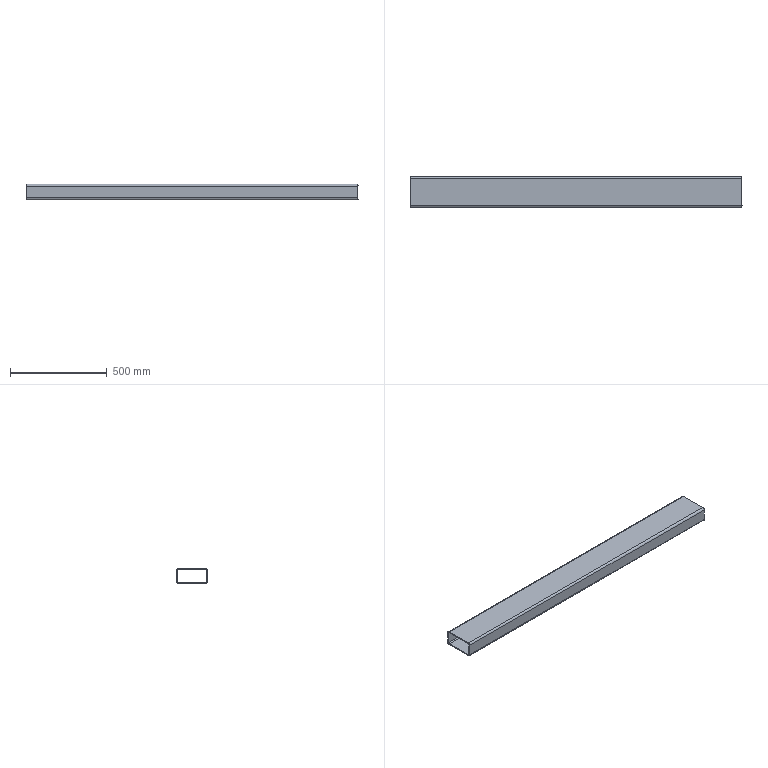Part | SolidWorks | features BaseBody 1 | 1 solid | 18 faces | box 1720 x 160 x 80 mm | volume 3845265 mm3 | plane 10 | cylinder 8 | commonest cylinder face diameters 10 x4 20 x4
STEP:
#1=CARTESIAN_POINT('',(-860.,70.,-40.));
#2=VERTEX_POINT('',#1);
#3=CARTESIAN_POINT('',(-860.,80.,-30.));
#4=VERTEX_POINT('',#3);
#5=CARTESIAN_POINT('',(-860.,70.,-30.));
#6=DIRECTION('',(1.,0.,0.));
#7=DIRECTION('',(0.,0.,-1.));
#8=AXIS2_PLACEMENT_3D('',#5,#6,#7);
#9=CIRCLE('',#8,10.);
#10=EDGE_CURVE('',#2,#4,#9,.T.);
#11=ORIENTED_EDGE('',*,*,#10,.T.);
#12=CARTESIAN_POINT('',(860.,80.,-30.));
#13=VERTEX_POINT('',#12);
#14=CARTESIAN_POINT('',(860.,80.,-30.));
#15=DIRECTION('',(-1.,0.,0.));
#16=VECTOR('',#15,1000.);
#17=LINE('',#14,#16);
#18=EDGE_CURVE('',#13,#4,#17,.T.);
#19=ORIENTED_EDGE('',*,*,#18,.F.);
#20=CARTESIAN_POINT('',(860.,70.,-40.));
#21=VERTEX_POINT('',#20);
#22=CARTESIAN_POINT('',(860.,70.,-30.));
#23=DIRECTION('',(1.,0.,0.));
#24=DIRECTION('',(0.,0.,-1.));
#25=AXIS2_PLACEMENT_3D('',#22,#23,#24);
#26=CIRCLE('',#25,10.);
#27=EDGE_CURVE('',#21,#13,#26,.T.);
#28=ORIENTED_EDGE('',*,*,#27,.F.);
#29=CARTESIAN_POINT('',(860.,70.,-40.));
#30=DIRECTION('',(-1.,0.,0.));
#31=VECTOR('',#30,1000.);
#32=LINE('',#29,#31);
#33=EDGE_CURVE('',#21,#2,#32,.T.);
#34=ORIENTED_EDGE('',*,*,#33,.T.);
#35=EDGE_LOOP('',(#11,#19,#28,#34));
#36=FACE_OUTER_BOUND('',#35,.T.);
#37=CARTESIAN_POINT('',(860.,70.,-30.));
#38=DIRECTION('',(-1.,0.,0.));
#39=DIRECTION('',(0.,0.,1.));
#40=AXIS2_PLACEMENT_3D('',#37,#38,#39);
#41=CYLINDRICAL_SURFACE('',#40,10.);
#42=ADVANCED_FACE('',(#36),#41,.T.);
#43=CARTESIAN_POINT('',(-860.,80.,30.));
#44=VERTEX_POINT('',#43);
#45=CARTESIAN_POINT('',(-860.,80.,-30.));
#46=DIRECTION('',(0.,0.,1.));
#47=VECTOR('',#46,1000.);
#48=LINE('',#45,#47);
#49=EDGE_CURVE('',#4,#44,#48,.T.);
#50=ORIENTED_EDGE('',*,*,#49,.T.);
#51=CARTESIAN_POINT('',(860.,80.,30.));
#52=VERTEX_POINT('',#51);
#53=CARTESIAN_POINT('',(860.,80.,30.));
#54=DIRECTION('',(-1.,0.,0.));
#55=VECTOR('',#54,1000.);
#56=LINE('',#53,#55);
#57=EDGE_CURVE('',#52,#44,#56,.T.);
#58=ORIENTED_EDGE('',*,*,#57,.F.);
#59=CARTESIAN_POINT('',(860.,80.,-30.));
#60=DIRECTION('',(0.,0.,1.));
#61=VECTOR('',#60,1000.);
#62=LINE('',#59,#61);
#63=EDGE_CURVE('',#13,#52,#62,.T.);
#64=ORIENTED_EDGE('',*,*,#63,.F.);
#65=ORIENTED_EDGE('',*,*,#18,.T.);
#66=EDGE_LOOP('',(#50,#58,#64,#65));
#67=FACE_OUTER_BOUND('',#66,.T.);
#68=CARTESIAN_POINT('',(860.,80.,-30.));
#69=DIRECTION('',(0.,-1.,0.));
#70=DIRECTION('',(0.,0.,-1.));
#71=AXIS2_PLACEMENT_3D('',#68,#69,#70);
#72=PLANE('',#71);
#73=ADVANCED_FACE('',(#67),#72,.F.);
#74=CARTESIAN_POINT('',(-860.,70.,40.));
#75=VERTEX_POINT('',#74);
#76=CARTESIAN_POINT('',(-860.,70.,30.));
#77=DIRECTION('',(1.,0.,0.));
#78=DIRECTION('',(0.,0.,-1.));
#79=AXIS2_PLACEMENT_3D('',#76,#77,#78);
#80=CIRCLE('',#79,10.);
#81=EDGE_CURVE('',#44,#75,#80,.T.);
#82=ORIENTED_EDGE('',*,*,#81,.T.);
#83=CARTESIAN_POINT('',(860.,70.,40.));
#84=VERTEX_POINT('',#83);
#85=CARTESIAN_POINT('',(860.,70.,40.));
#86=DIRECTION('',(-1.,0.,0.));
#87=VECTOR('',#86,1000.);
#88=LINE('',#85,#87);
#89=EDGE_CURVE('',#84,#75,#88,.T.);
#90=ORIENTED_EDGE('',*,*,#89,.F.);
#91=CARTESIAN_POINT('',(860.,70.,30.));
#92=DIRECTION('',(1.,0.,0.));
#93=DIRECTION('',(0.,0.,-1.));
#94=AXIS2_PLACEMENT_3D('',#91,#92,#93);
#95=CIRCLE('',#94,10.);
#96=EDGE_CURVE('',#52,#84,#95,.T.);
#97=ORIENTED_EDGE('',*,*,#96,.F.);
#98=ORIENTED_EDGE('',*,*,#57,.T.);
#99=EDGE_LOOP('',(#82,#90,#97,#98));
#100=FACE_OUTER_BOUND('',#99,.T.);
#101=CARTESIAN_POINT('',(860.,70.,30.));
#102=DIRECTION('',(-1.,0.,0.));
#103=DIRECTION('',(0.,0.,1.));
#104=AXIS2_PLACEMENT_3D('',#101,#102,#103);
#105=CYLINDRICAL_SURFACE('',#104,10.);
#106=ADVANCED_FACE('',(#100),#105,.T.);
#107=CARTESIAN_POINT('',(-860.,-70.,40.));
#108=VERTEX_POINT('',#107);
#109=CARTESIAN_POINT('',(-860.,-70.,40.));
#110=DIRECTION('',(0.,-1.,0.));
#111=VECTOR('',#110,1000.);
#112=LINE('',#109,#111);
#113=EDGE_CURVE('',#75,#108,#112,.T.);
#114=ORIENTED_EDGE('',*,*,#113,.T.);
#115=CARTESIAN_POINT('',(860.,-70.,40.));
#116=VERTEX_POINT('',#115);
#117=CARTESIAN_POINT('',(860.,-70.,40.));
#118=DIRECTION('',(-1.,0.,0.));
#119=VECTOR('',#118,1000.);
#120=LINE('',#117,#119);
#121=EDGE_CURVE('',#116,#108,#120,.T.);
#122=ORIENTED_EDGE('',*,*,#121,.F.);
#123=CARTESIAN_POINT('',(860.,-70.,40.));
#124=DIRECTION('',(0.,-1.,0.));
#125=VECTOR('',#124,1000.);
#126=LINE('',#123,#125);
#127=EDGE_CURVE('',#84,#116,#126,.T.);
#128=ORIENTED_EDGE('',*,*,#127,.F.);
#129=ORIENTED_EDGE('',*,*,#89,.T.);
#130=EDGE_LOOP('',(#114,#122,#128,#129));
#131=FACE_OUTER_BOUND('',#130,.T.);
#132=CARTESIAN_POINT('',(860.,-70.,40.));
#133=DIRECTION('',(0.,0.,-1.));
#134=DIRECTION('',(0.,1.,0.));
#135=AXIS2_PLACEMENT_3D('',#132,#133,#134);
#136=PLANE('',#135);
#137=ADVANCED_FACE('',(#131),#136,.F.);
#138=CARTESIAN_POINT('',(-860.,-80.,30.));
#139=VERTEX_POINT('',#138);
#140=CARTESIAN_POINT('',(-860.,-70.,30.));
#141=DIRECTION('',(1.,0.,0.));
#142=DIRECTION('',(0.,0.,-1.));
#143=AXIS2_PLACEMENT_3D('',#140,#141,#142);
#144=CIRCLE('',#143,10.);
#145=EDGE_CURVE('',#108,#139,#144,.T.);
#146=ORIENTED_EDGE('',*,*,#145,.T.);
#147=CARTESIAN_POINT('',(860.,-80.,30.));
#148=VERTEX_POINT('',#147);
#149=CARTESIAN_POINT('',(860.,-80.,30.));
#150=DIRECTION('',(-1.,0.,0.));
#151=VECTOR('',#150,1000.);
#152=LINE('',#149,#151);
#153=EDGE_CURVE('',#148,#139,#152,.T.);
#154=ORIENTED_EDGE('',*,*,#153,.F.);
#155=CARTESIAN_POINT('',(860.,-70.,30.));
#156=DIRECTION('',(1.,0.,0.));
#157=DIRECTION('',(0.,0.,-1.));
#158=AXIS2_PLACEMENT_3D('',#155,#156,#157);
#159=CIRCLE('',#158,10.);
#160=EDGE_CURVE('',#116,#148,#159,.T.);
#161=ORIENTED_EDGE('',*,*,#160,.F.);
#162=ORIENTED_EDGE('',*,*,#121,.T.);
#163=EDGE_LOOP('',(#146,#154,#161,#162));
#164=FACE_OUTER_BOUND('',#163,.T.);
#165=CARTESIAN_POINT('',(860.,-70.,30.));
#166=DIRECTION('',(-1.,0.,0.));
#167=DIRECTION('',(0.,0.,1.));
#168=AXIS2_PLACEMENT_3D('',#165,#166,#167);
#169=CYLINDRICAL_SURFACE('',#168,10.);
#170=ADVANCED_FACE('',(#164),#169,.T.);
#171=CARTESIAN_POINT('',(-860.,-80.,-30.));
#172=VERTEX_POINT('',#171);
#173=CARTESIAN_POINT('',(-860.,-80.,30.));
#174=DIRECTION('',(0.,0.,-1.));
#175=VECTOR('',#174,1000.);
#176=LINE('',#173,#175);
#177=EDGE_CURVE('',#139,#172,#176,.T.);
#178=ORIENTED_EDGE('',*,*,#177,.T.);
#179=CARTESIAN_POINT('',(860.,-80.,-30.));
#180=VERTEX_POINT('',#179);
#181=CARTESIAN_POINT('',(860.,-80.,-30.));
#182=DIRECTION('',(-1.,0.,0.));
#183=VECTOR('',#182,1000.);
#184=LINE('',#181,#183);
#185=EDGE_CURVE('',#180,#172,#184,.T.);
#186=ORIENTED_EDGE('',*,*,#185,.F.);
#187=CARTESIAN_POINT('',(860.,-80.,30.));
#188=DIRECTION('',(0.,0.,-1.));
#189=VECTOR('',#188,1000.);
#190=LINE('',#187,#189);
#191=EDGE_CURVE('',#148,#180,#190,.T.);
#192=ORIENTED_EDGE('',*,*,#191,.F.);
#193=ORIENTED_EDGE('',*,*,#153,.T.);
#194=EDGE_LOOP('',(#178,#186,#192,#193));
#195=FACE_OUTER_BOUND('',#194,.T.);
#196=CARTESIAN_POINT('',(860.,-80.,30.));
#197=DIRECTION('',(0.,1.,0.));
#198=DIRECTION('',(0.,0.,1.));
#199=AXIS2_PLACEMENT_3D('',#196,#197,#198);
#200=PLANE('',#199);
#201=ADVANCED_FACE('',(#195),#200,.F.);
#202=CARTESIAN_POINT('',(-860.,-70.,-40.));
#203=VERTEX_POINT('',#202);
#204=CARTESIAN_POINT('',(-860.,-70.,-30.));
#205=DIRECTION('',(1.,0.,0.));
#206=DIRECTION('',(0.,0.,-1.));
#207=AXIS2_PLACEMENT_3D('',#204,#205,#206);
#208=CIRCLE('',#207,10.);
#209=EDGE_CURVE('',#172,#203,#208,.T.);
#210=ORIENTED_EDGE('',*,*,#209,.T.);
#211=CARTESIAN_POINT('',(860.,-70.,-40.));
#212=VERTEX_POINT('',#211);
#213=CARTESIAN_POINT('',(860.,-70.,-40.));
#214=DIRECTION('',(-1.,0.,0.));
#215=VECTOR('',#214,1000.);
#216=LINE('',#213,#215);
#217=EDGE_CURVE('',#212,#203,#216,.T.);
#218=ORIENTED_EDGE('',*,*,#217,.F.);
#219=CARTESIAN_POINT('',(860.,-70.,-30.));
#220=DIRECTION('',(1.,0.,0.));
#221=DIRECTION('',(0.,0.,-1.));
#222=AXIS2_PLACEMENT_3D('',#219,#220,#221);
#223=CIRCLE('',#222,10.);
#224=EDGE_CURVE('',#180,#212,#223,.T.);
#225=ORIENTED_EDGE('',*,*,#224,.F.);
#226=ORIENTED_EDGE('',*,*,#185,.T.);
#227=EDGE_LOOP('',(#210,#218,#225,#226));
#228=FACE_OUTER_BOUND('',#227,.T.);
#229=CARTESIAN_POINT('',(860.,-70.,-30.));
#230=DIRECTION('',(-1.,0.,0.));
#231=DIRECTION('',(0.,0.,1.));
#232=AXIS2_PLACEMENT_3D('',#229,#230,#231);
#233=CYLINDRICAL_SURFACE('',#232,10.);
#234=ADVANCED_FACE('',(#228),#233,.T.);
#235=CARTESIAN_POINT('',(-860.,75.,30.));
#236=VERTEX_POINT('',#235);
#237=CARTESIAN_POINT('',(-860.,70.,35.));
#238=VERTEX_POINT('',#237);
#239=CARTESIAN_POINT('',(-860.,70.,30.));
#240=DIRECTION('',(1.,0.,0.));
#241=DIRECTION('',(0.,0.,-1.));
#242=AXIS2_PLACEMENT_3D('',#239,#240,#241);
#243=CIRCLE('',#242,5.);
#244=EDGE_CURVE('',#236,#238,#243,.T.);
#245=ORIENTED_EDGE('',*,*,#244,.F.);
#246=CARTESIAN_POINT('',(860.,75.,30.));
#247=VERTEX_POINT('',#246);
#248=CARTESIAN_POINT('',(860.,75.,30.));
#249=DIRECTION('',(-1.,0.,0.));
#250=VECTOR('',#249,1000.);
#251=LINE('',#248,#250);
#252=EDGE_CURVE('',#247,#236,#251,.T.);
#253=ORIENTED_EDGE('',*,*,#252,.F.);
#254=CARTESIAN_POINT('',(860.,70.,35.));
#255=VERTEX_POINT('',#254);
#256=CARTESIAN_POINT('',(860.,70.,30.));
#257=DIRECTION('',(1.,0.,0.));
#258=DIRECTION('',(0.,0.,-1.));
#259=AXIS2_PLACEMENT_3D('',#256,#257,#258);
#260=CIRCLE('',#259,5.);
#261=EDGE_CURVE('',#247,#255,#260,.T.);
#262=ORIENTED_EDGE('',*,*,#261,.T.);
#263=CARTESIAN_POINT('',(860.,70.,35.));
#264=DIRECTION('',(-1.,0.,0.));
#265=VECTOR('',#264,1000.);
#266=LINE('',#263,#265);
#267=EDGE_CURVE('',#255,#238,#266,.T.);
#268=ORIENTED_EDGE('',*,*,#267,.T.);
#269=EDGE_LOOP('',(#245,#253,#262,#268));
#270=FACE_OUTER_BOUND('',#269,.T.);
#271=CARTESIAN_POINT('',(860.,70.,30.));
#272=DIRECTION('',(-1.,0.,0.));
#273=DIRECTION('',(0.,0.,1.));
#274=AXIS2_PLACEMENT_3D('',#271,#272,#273);
#275=CYLINDRICAL_SURFACE('',#274,5.);
#276=ADVANCED_FACE('',(#270),#275,.F.);
#277=CARTESIAN_POINT('',(-860.,75.,-30.));
#278=VERTEX_POINT('',#277);
#279=CARTESIAN_POINT('',(-860.,75.,-30.));
#280=DIRECTION('',(0.,0.,1.));
#281=VECTOR('',#280,1000.);
#282=LINE('',#279,#281);
#283=EDGE_CURVE('',#278,#236,#282,.T.);
#284=ORIENTED_EDGE('',*,*,#283,.F.);
#285=CARTESIAN_POINT('',(860.,75.,-30.));
#286=VERTEX_POINT('',#285);
#287=CARTESIAN_POINT('',(860.,75.,-30.));
#288=DIRECTION('',(-1.,0.,0.));
#289=VECTOR('',#288,1000.);
#290=LINE('',#287,#289);
#291=EDGE_CURVE('',#286,#278,#290,.T.);
#292=ORIENTED_EDGE('',*,*,#291,.F.);
#293=CARTESIAN_POINT('',(860.,75.,-30.));
#294=DIRECTION('',(0.,0.,1.));
#295=VECTOR('',#294,1000.);
#296=LINE('',#293,#295);
#297=EDGE_CURVE('',#286,#247,#296,.T.);
#298=ORIENTED_EDGE('',*,*,#297,.T.);
#299=ORIENTED_EDGE('',*,*,#252,.T.);
#300=EDGE_LOOP('',(#284,#292,#298,#299));
#301=FACE_OUTER_BOUND('',#300,.T.);
#302=CARTESIAN_POINT('',(860.,75.,-30.));
#303=DIRECTION('',(0.,-1.,0.));
#304=DIRECTION('',(0.,0.,-1.));
#305=AXIS2_PLACEMENT_3D('',#302,#303,#304);
#306=PLANE('',#305);
#307=ADVANCED_FACE('',(#301),#306,.T.);
#308=CARTESIAN_POINT('',(-860.,70.,-35.));
#309=VERTEX_POINT('',#308);
#310=CARTESIAN_POINT('',(-860.,70.,-30.));
#311=DIRECTION('',(1.,0.,0.));
#312=DIRECTION('',(0.,0.,-1.));
#313=AXIS2_PLACEMENT_3D('',#310,#311,#312);
#314=CIRCLE('',#313,5.);
#315=EDGE_CURVE('',#309,#278,#314,.T.);
#316=ORIENTED_EDGE('',*,*,#315,.F.);
#317=CARTESIAN_POINT('',(860.,70.,-35.));
#318=VERTEX_POINT('',#317);
#319=CARTESIAN_POINT('',(860.,70.,-35.));
#320=DIRECTION('',(-1.,0.,0.));
#321=VECTOR('',#320,1000.);
#322=LINE('',#319,#321);
#323=EDGE_CURVE('',#318,#309,#322,.T.);
#324=ORIENTED_EDGE('',*,*,#323,.F.);
#325=CARTESIAN_POINT('',(860.,70.,-30.));
#326=DIRECTION('',(1.,0.,0.));
#327=DIRECTION('',(0.,0.,-1.));
#328=AXIS2_PLACEMENT_3D('',#325,#326,#327);
#329=CIRCLE('',#328,5.);
#330=EDGE_CURVE('',#318,#286,#329,.T.);
#331=ORIENTED_EDGE('',*,*,#330,.T.);
#332=ORIENTED_EDGE('',*,*,#291,.T.);
#333=EDGE_LOOP('',(#316,#324,#331,#332));
#334=FACE_OUTER_BOUND('',#333,.T.);
#335=CARTESIAN_POINT('',(860.,70.,-30.));
#336=DIRECTION('',(-1.,0.,0.));
#337=DIRECTION('',(0.,0.,1.));
#338=AXIS2_PLACEMENT_3D('',#335,#336,#337);
#339=CYLINDRICAL_SURFACE('',#338,5.);
#340=ADVANCED_FACE('',(#334),#339,.F.);
#341=CARTESIAN_POINT('',(-860.,-70.,-35.));
#342=VERTEX_POINT('',#341);
#343=CARTESIAN_POINT('',(-860.,70.,-35.));
#344=DIRECTION('',(0.,1.,0.));
#345=VECTOR('',#344,1000.);
#346=LINE('',#343,#345);
#347=EDGE_CURVE('',#342,#309,#346,.T.);
#348=ORIENTED_EDGE('',*,*,#347,.F.);
#349=CARTESIAN_POINT('',(860.,-70.,-35.));
#350=VERTEX_POINT('',#349);
#351=CARTESIAN_POINT('',(860.,-70.,-35.));
#352=DIRECTION('',(-1.,0.,0.));
#353=VECTOR('',#352,1000.);
#354=LINE('',#351,#353);
#355=EDGE_CURVE('',#350,#342,#354,.T.);
#356=ORIENTED_EDGE('',*,*,#355,.F.);
#357=CARTESIAN_POINT('',(860.,70.,-35.));
#358=DIRECTION('',(0.,1.,0.));
#359=VECTOR('',#358,1000.);
#360=LINE('',#357,#359);
#361=EDGE_CURVE('',#350,#318,#360,.T.);
#362=ORIENTED_EDGE('',*,*,#361,.T.);
#363=ORIENTED_EDGE('',*,*,#323,.T.);
#364=EDGE_LOOP('',(#348,#356,#362,#363));
#365=FACE_OUTER_BOUND('',#364,.T.);
#366=CARTESIAN_POINT('',(860.,70.,-35.));
#367=DIRECTION('',(0.,0.,1.));
#368=DIRECTION('',(1.,0.,0.));
#369=AXIS2_PLACEMENT_3D('',#366,#367,#368);
#370=PLANE('',#369);
#371=ADVANCED_FACE('',(#365),#370,.T.);
#372=CARTESIAN_POINT('',(-860.,-75.,-30.));
#373=VERTEX_POINT('',#372);
#374=CARTESIAN_POINT('',(-860.,-70.,-30.));
#375=DIRECTION('',(1.,0.,0.));
#376=DIRECTION('',(0.,0.,-1.));
#377=AXIS2_PLACEMENT_3D('',#374,#375,#376);
#378=CIRCLE('',#377,5.);
#379=EDGE_CURVE('',#373,#342,#378,.T.);
#380=ORIENTED_EDGE('',*,*,#379,.F.);
#381=CARTESIAN_POINT('',(860.,-75.,-30.));
#382=VERTEX_POINT('',#381);
#383=CARTESIAN_POINT('',(860.,-75.,-30.));
#384=DIRECTION('',(-1.,0.,0.));
#385=VECTOR('',#384,1000.);
#386=LINE('',#383,#385);
#387=EDGE_CURVE('',#382,#373,#386,.T.);
#388=ORIENTED_EDGE('',*,*,#387,.F.);
#389=CARTESIAN_POINT('',(860.,-70.,-30.));
#390=DIRECTION('',(1.,0.,0.));
#391=DIRECTION('',(0.,0.,-1.));
#392=AXIS2_PLACEMENT_3D('',#389,#390,#391);
#393=CIRCLE('',#392,5.);
#394=EDGE_CURVE('',#382,#350,#393,.T.);
#395=ORIENTED_EDGE('',*,*,#394,.T.);
#396=ORIENTED_EDGE('',*,*,#355,.T.);
#397=EDGE_LOOP('',(#380,#388,#395,#396));
#398=FACE_OUTER_BOUND('',#397,.T.);
#399=CARTESIAN_POINT('',(860.,-70.,-30.));
#400=DIRECTION('',(-1.,0.,0.));
#401=DIRECTION('',(0.,0.,1.));
#402=AXIS2_PLACEMENT_3D('',#399,#400,#401);
#403=CYLINDRICAL_SURFACE('',#402,5.);
#404=ADVANCED_FACE('',(#398),#403,.F.);
#405=CARTESIAN_POINT('',(-860.,-75.,30.));
#406=VERTEX_POINT('',#405);
#407=CARTESIAN_POINT('',(-860.,-75.,30.));
#408=DIRECTION('',(0.,0.,-1.));
#409=VECTOR('',#408,1000.);
#410=LINE('',#407,#409);
#411=EDGE_CURVE('',#406,#373,#410,.T.);
#412=ORIENTED_EDGE('',*,*,#411,.F.);
#413=CARTESIAN_POINT('',(860.,-75.,30.));
#414=VERTEX_POINT('',#413);
#415=CARTESIAN_POINT('',(860.,-75.,30.));
#416=DIRECTION('',(-1.,0.,0.));
#417=VECTOR('',#416,1000.);
#418=LINE('',#415,#417);
#419=EDGE_CURVE('',#414,#406,#418,.T.);
#420=ORIENTED_EDGE('',*,*,#419,.F.);
#421=CARTESIAN_POINT('',(860.,-75.,30.));
#422=DIRECTION('',(0.,0.,-1.));
#423=VECTOR('',#422,1000.);
#424=LINE('',#421,#423);
#425=EDGE_CURVE('',#414,#382,#424,.T.);
#426=ORIENTED_EDGE('',*,*,#425,.T.);
#427=ORIENTED_EDGE('',*,*,#387,.T.);
#428=EDGE_LOOP('',(#412,#420,#426,#427));
#429=FACE_OUTER_BOUND('',#428,.T.);
#430=CARTESIAN_POINT('',(860.,-75.,30.));
#431=DIRECTION('',(0.,1.,0.));
#432=DIRECTION('',(0.,0.,1.));
#433=AXIS2_PLACEMENT_3D('',#430,#431,#432);
#434=PLANE('',#433);
#435=ADVANCED_FACE('',(#429),#434,.T.);
#436=CARTESIAN_POINT('',(-860.,-70.,35.));
#437=VERTEX_POINT('',#436);
#438=CARTESIAN_POINT('',(-860.,-70.,30.));
#439=DIRECTION('',(1.,0.,0.));
#440=DIRECTION('',(0.,0.,-1.));
#441=AXIS2_PLACEMENT_3D('',#438,#439,#440);
#442=CIRCLE('',#441,5.);
#443=EDGE_CURVE('',#437,#406,#442,.T.);
#444=ORIENTED_EDGE('',*,*,#443,.F.);
#445=CARTESIAN_POINT('',(860.,-70.,35.));
#446=VERTEX_POINT('',#445);
#447=CARTESIAN_POINT('',(860.,-70.,35.));
#448=DIRECTION('',(-1.,0.,0.));
#449=VECTOR('',#448,1000.);
#450=LINE('',#447,#449);
#451=EDGE_CURVE('',#446,#437,#450,.T.);
#452=ORIENTED_EDGE('',*,*,#451,.F.);
#453=CARTESIAN_POINT('',(860.,-70.,30.));
#454=DIRECTION('',(1.,0.,0.));
#455=DIRECTION('',(0.,0.,-1.));
#456=AXIS2_PLACEMENT_3D('',#453,#454,#455);
#457=CIRCLE('',#456,5.);
#458=EDGE_CURVE('',#446,#414,#457,.T.);
#459=ORIENTED_EDGE('',*,*,#458,.T.);
#460=ORIENTED_EDGE('',*,*,#419,.T.);
#461=EDGE_LOOP('',(#444,#452,#459,#460));
#462=FACE_OUTER_BOUND('',#461,.T.);
#463=CARTESIAN_POINT('',(860.,-70.,30.));
#464=DIRECTION('',(-1.,0.,0.));
#465=DIRECTION('',(0.,0.,1.));
#466=AXIS2_PLACEMENT_3D('',#463,#464,#465);
#467=CYLINDRICAL_SURFACE('',#466,5.);
#468=ADVANCED_FACE('',(#462),#467,.F.);
#469=CARTESIAN_POINT('',(-860.,-70.,35.));
#470=DIRECTION('',(0.,-1.,0.));
#471=VECTOR('',#470,1000.);
#472=LINE('',#469,#471);
#473=EDGE_CURVE('',#238,#437,#472,.T.);
#474=ORIENTED_EDGE('',*,*,#473,.F.);
#475=ORIENTED_EDGE('',*,*,#267,.F.);
#476=CARTESIAN_POINT('',(860.,-70.,35.));
#477=DIRECTION('',(0.,-1.,0.));
#478=VECTOR('',#477,1000.);
#479=LINE('',#476,#478);
#480=EDGE_CURVE('',#255,#446,#479,.T.);
#481=ORIENTED_EDGE('',*,*,#480,.T.);
#482=ORIENTED_EDGE('',*,*,#451,.T.);
#483=EDGE_LOOP('',(#474,#475,#481,#482));
#484=FACE_OUTER_BOUND('',#483,.T.);
#485=CARTESIAN_POINT('',(860.,-70.,35.));
#486=DIRECTION('',(0.,0.,-1.));
#487=DIRECTION('',(0.,1.,0.));
#488=AXIS2_PLACEMENT_3D('',#485,#486,#487);
#489=PLANE('',#488);
#490=ADVANCED_FACE('',(#484),#489,.T.);
#491=CARTESIAN_POINT('',(-860.,70.,-40.));
#492=DIRECTION('',(0.,1.,0.));
#493=VECTOR('',#492,1000.);
#494=LINE('',#491,#493);
#495=EDGE_CURVE('',#203,#2,#494,.T.);
#496=ORIENTED_EDGE('',*,*,#495,.T.);
#497=ORIENTED_EDGE('',*,*,#33,.F.);
#498=CARTESIAN_POINT('',(860.,70.,-40.));
#499=DIRECTION('',(0.,1.,0.));
#500=VECTOR('',#499,1000.);
#501=LINE('',#498,#500);
#502=EDGE_CURVE('',#212,#21,#501,.T.);
#503=ORIENTED_EDGE('',*,*,#502,.F.);
#504=ORIENTED_EDGE('',*,*,#217,.T.);
#505=EDGE_LOOP('',(#496,#497,#503,#504));
#506=FACE_OUTER_BOUND('',#505,.T.);
#507=CARTESIAN_POINT('',(860.,70.,-40.));
#508=DIRECTION('',(0.,0.,1.));
#509=DIRECTION('',(1.,0.,0.));
#510=AXIS2_PLACEMENT_3D('',#507,#508,#509);
#511=PLANE('',#510);
#512=ADVANCED_FACE('',(#506),#511,.F.);
#513=ORIENTED_EDGE('',*,*,#261,.F.);
#514=ORIENTED_EDGE('',*,*,#297,.F.);
#515=ORIENTED_EDGE('',*,*,#330,.F.);
#516=ORIENTED_EDGE('',*,*,#361,.F.);
#517=ORIENTED_EDGE('',*,*,#394,.F.);
#518=ORIENTED_EDGE('',*,*,#425,.F.);
#519=ORIENTED_EDGE('',*,*,#458,.F.);
#520=ORIENTED_EDGE('',*,*,#480,.F.);
#521=EDGE_LOOP('',(#513,#514,#515,#516,#517,#518,#519,#520));
#522=FACE_BOUND('',#521,.T.);
#523=ORIENTED_EDGE('',*,*,#27,.T.);
#524=ORIENTED_EDGE('',*,*,#63,.T.);
#525=ORIENTED_EDGE('',*,*,#96,.T.);
#526=ORIENTED_EDGE('',*,*,#127,.T.);
#527=ORIENTED_EDGE('',*,*,#160,.T.);
#528=ORIENTED_EDGE('',*,*,#191,.T.);
#529=ORIENTED_EDGE('',*,*,#224,.T.);
#530=ORIENTED_EDGE('',*,*,#502,.T.);
#531=EDGE_LOOP('',(#523,#524,#525,#526,#527,#528,#529,#530));
#532=FACE_OUTER_BOUND('',#531,.T.);
#533=CARTESIAN_POINT('',(860.,70.,-30.));
#534=DIRECTION('',(1.,0.,0.));
#535=DIRECTION('',(0.,0.,-1.));
#536=AXIS2_PLACEMENT_3D('',#533,#534,#535);
#537=PLANE('',#536);
#538=ADVANCED_FACE('',(#522,#532),#537,.T.);
#539=ORIENTED_EDGE('',*,*,#244,.T.);
#540=ORIENTED_EDGE('',*,*,#473,.T.);
#541=ORIENTED_EDGE('',*,*,#443,.T.);
#542=ORIENTED_EDGE('',*,*,#411,.T.);
#543=ORIENTED_EDGE('',*,*,#379,.T.);
#544=ORIENTED_EDGE('',*,*,#347,.T.);
#545=ORIENTED_EDGE('',*,*,#315,.T.);
#546=ORIENTED_EDGE('',*,*,#283,.T.);
#547=EDGE_LOOP('',(#539,#540,#541,#542,#543,#544,#545,#546));
#548=FACE_BOUND('',#547,.T.);
#549=ORIENTED_EDGE('',*,*,#10,.F.);
#550=ORIENTED_EDGE('',*,*,#495,.F.);
#551=ORIENTED_EDGE('',*,*,#209,.F.);
#552=ORIENTED_EDGE('',*,*,#177,.F.);
#553=ORIENTED_EDGE('',*,*,#145,.F.);
#554=ORIENTED_EDGE('',*,*,#113,.F.);
#555=ORIENTED_EDGE('',*,*,#81,.F.);
#556=ORIENTED_EDGE('',*,*,#49,.F.);
#557=EDGE_LOOP('',(#549,#550,#551,#552,#553,#554,#555,#556));
#558=FACE_OUTER_BOUND('',#557,.T.);
#559=CARTESIAN_POINT('',(-860.,70.,-30.));
#560=DIRECTION('',(1.,0.,0.));
#561=DIRECTION('',(0.,0.,-1.));
#562=AXIS2_PLACEMENT_3D('',#559,#560,#561);
#563=PLANE('',#562);
#564=ADVANCED_FACE('',(#548,#558),#563,.F.);
#565=CLOSED_SHELL('',(#42,#73,#106,#137,#170,#201,#234,#276,#307,#340,#371,#404,#435,#468,#490,#512,#538,#564));
#566=MANIFOLD_SOLID_BREP('',#565);
#567=CARTESIAN_POINT('',(0.,0.,0.));
#568=DIRECTION('',(0.,0.,1.));
#569=DIRECTION('',(1.,0.,0.));
#570=AXIS2_PLACEMENT_3D('',#567,#568,#569);
#571=(LENGTH_UNIT()NAMED_UNIT(*)SI_UNIT(.MILLI.,.METRE.));
#572=UNCERTAINTY_MEASURE_WITH_UNIT(LENGTH_MEASURE(0.00001),#571,'','');
#573=(NAMED_UNIT(*)PLANE_ANGLE_UNIT()SI_UNIT($,.RADIAN.));
#574=(NAMED_UNIT(*)SI_UNIT($,.STERADIAN.)SOLID_ANGLE_UNIT());
#575=(GEOMETRIC_REPRESENTATION_CONTEXT(3)GLOBAL_UNCERTAINTY_ASSIGNED_CONTEXT((#572))GLOBAL_UNIT_ASSIGNED_CONTEXT((#571,#573,#574))REPRESENTATION_CONTEXT('',''));
#576=ADVANCED_BREP_SHAPE_REPRESENTATION('',(#566,#570),#575);